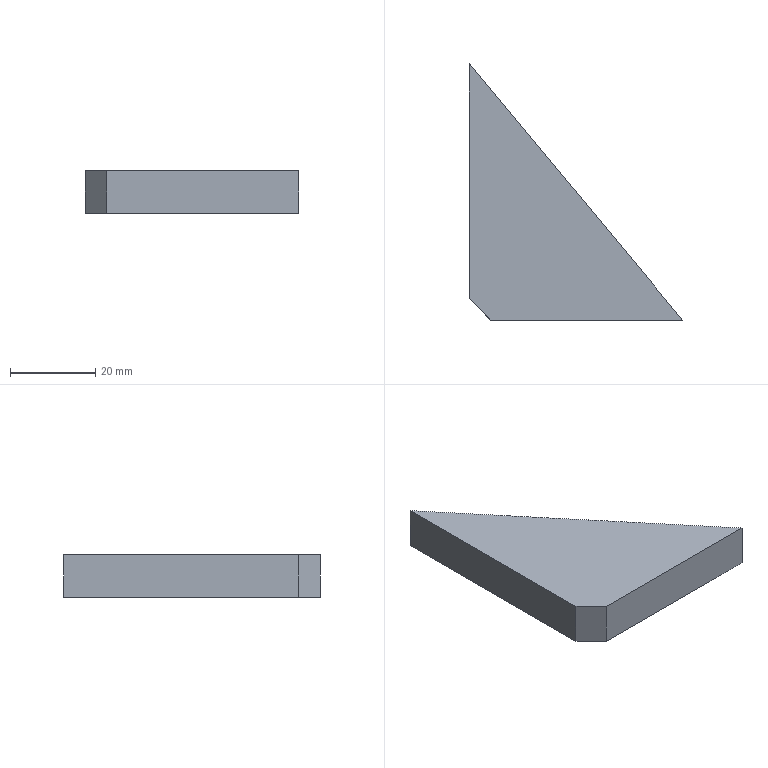Part | SolidWorks | features Chamfer 1, Extrusion 1 | 1 solid | 6 faces | box 50 x 60 x 10 mm | volume 14875 mm3 | plane 6
STEP:
#1=CARTESIAN_POINT('',(5.,0.,5.));
#2=VERTEX_POINT('',#1);
#3=CARTESIAN_POINT('',(50.,0.,5.));
#4=VERTEX_POINT('',#3);
#5=CARTESIAN_POINT('',(50.,0.,5.));
#6=DIRECTION('',(1.,0.,0.));
#7=VECTOR('',#6,1000.);
#8=LINE('',#5,#7);
#9=EDGE_CURVE('',#2,#4,#8,.T.);
#10=ORIENTED_EDGE('',*,*,#9,.F.);
#11=CARTESIAN_POINT('',(5.,0.,-5.));
#12=VERTEX_POINT('',#11);
#13=CARTESIAN_POINT('',(5.,0.,5.));
#14=DIRECTION('',(0.,0.,-1.));
#15=VECTOR('',#14,1000.);
#16=LINE('',#13,#15);
#17=EDGE_CURVE('',#2,#12,#16,.T.);
#18=ORIENTED_EDGE('',*,*,#17,.T.);
#19=CARTESIAN_POINT('',(50.,0.,-5.));
#20=VERTEX_POINT('',#19);
#21=CARTESIAN_POINT('',(50.,0.,-5.));
#22=DIRECTION('',(1.,0.,0.));
#23=VECTOR('',#22,1000.);
#24=LINE('',#21,#23);
#25=EDGE_CURVE('',#12,#20,#24,.T.);
#26=ORIENTED_EDGE('',*,*,#25,.T.);
#27=CARTESIAN_POINT('',(50.,0.,5.));
#28=DIRECTION('',(0.,0.,-1.));
#29=VECTOR('',#28,1000.);
#30=LINE('',#27,#29);
#31=EDGE_CURVE('',#4,#20,#30,.T.);
#32=ORIENTED_EDGE('',*,*,#31,.F.);
#33=EDGE_LOOP('',(#10,#18,#26,#32));
#34=FACE_OUTER_BOUND('',#33,.T.);
#35=CARTESIAN_POINT('',(50.,0.,5.));
#36=DIRECTION('',(0.,1.,0.));
#37=DIRECTION('',(0.,0.,1.));
#38=AXIS2_PLACEMENT_3D('',#35,#36,#37);
#39=PLANE('',#38);
#40=ADVANCED_FACE('',(#34),#39,.F.);
#41=CARTESIAN_POINT('',(0.,60.,-5.));
#42=VERTEX_POINT('',#41);
#43=CARTESIAN_POINT('',(0.,60.,-5.));
#44=DIRECTION('',(-0.6402,0.7682,0.));
#45=VECTOR('',#44,1000.);
#46=LINE('',#43,#45);
#47=EDGE_CURVE('',#20,#42,#46,.T.);
#48=ORIENTED_EDGE('',*,*,#47,.T.);
#49=CARTESIAN_POINT('',(0.,60.,5.));
#50=VERTEX_POINT('',#49);
#51=CARTESIAN_POINT('',(0.,60.,5.));
#52=DIRECTION('',(0.,0.,-1.));
#53=VECTOR('',#52,1000.);
#54=LINE('',#51,#53);
#55=EDGE_CURVE('',#50,#42,#54,.T.);
#56=ORIENTED_EDGE('',*,*,#55,.F.);
#57=CARTESIAN_POINT('',(0.,60.,5.));
#58=DIRECTION('',(-0.6402,0.7682,0.));
#59=VECTOR('',#58,1000.);
#60=LINE('',#57,#59);
#61=EDGE_CURVE('',#4,#50,#60,.T.);
#62=ORIENTED_EDGE('',*,*,#61,.F.);
#63=ORIENTED_EDGE('',*,*,#31,.T.);
#64=EDGE_LOOP('',(#48,#56,#62,#63));
#65=FACE_OUTER_BOUND('',#64,.T.);
#66=CARTESIAN_POINT('',(0.,60.,5.));
#67=DIRECTION('',(-0.7682,-0.6402,0.));
#68=DIRECTION('',(0.6402,-0.7682,0.));
#69=AXIS2_PLACEMENT_3D('',#66,#67,#68);
#70=PLANE('',#69);
#71=ADVANCED_FACE('',(#65),#70,.F.);
#72=CARTESIAN_POINT('',(0.,5.,-5.));
#73=VERTEX_POINT('',#72);
#74=CARTESIAN_POINT('',(0.,0.,-5.));
#75=DIRECTION('',(0.,-1.,0.));
#76=VECTOR('',#75,1000.);
#77=LINE('',#74,#76);
#78=EDGE_CURVE('',#42,#73,#77,.T.);
#79=ORIENTED_EDGE('',*,*,#78,.T.);
#80=CARTESIAN_POINT('',(0.,5.,5.));
#81=VERTEX_POINT('',#80);
#82=CARTESIAN_POINT('',(0.,5.,5.));
#83=DIRECTION('',(0.,0.,1.));
#84=VECTOR('',#83,1000.);
#85=LINE('',#82,#84);
#86=EDGE_CURVE('',#73,#81,#85,.T.);
#87=ORIENTED_EDGE('',*,*,#86,.T.);
#88=CARTESIAN_POINT('',(0.,0.,5.));
#89=DIRECTION('',(0.,-1.,0.));
#90=VECTOR('',#89,1000.);
#91=LINE('',#88,#90);
#92=EDGE_CURVE('',#50,#81,#91,.T.);
#93=ORIENTED_EDGE('',*,*,#92,.F.);
#94=ORIENTED_EDGE('',*,*,#55,.T.);
#95=EDGE_LOOP('',(#79,#87,#93,#94));
#96=FACE_OUTER_BOUND('',#95,.T.);
#97=CARTESIAN_POINT('',(0.,0.,5.));
#98=DIRECTION('',(1.,0.,0.));
#99=DIRECTION('',(0.,0.,-1.));
#100=AXIS2_PLACEMENT_3D('',#97,#98,#99);
#101=PLANE('',#100);
#102=ADVANCED_FACE('',(#96),#101,.F.);
#103=ORIENTED_EDGE('',*,*,#92,.T.);
#104=CARTESIAN_POINT('',(5.,0.,5.));
#105=DIRECTION('',(0.7071,-0.7071,0.));
#106=VECTOR('',#105,1000.);
#107=LINE('',#104,#106);
#108=EDGE_CURVE('',#81,#2,#107,.T.);
#109=ORIENTED_EDGE('',*,*,#108,.T.);
#110=ORIENTED_EDGE('',*,*,#9,.T.);
#111=ORIENTED_EDGE('',*,*,#61,.T.);
#112=EDGE_LOOP('',(#103,#109,#110,#111));
#113=FACE_OUTER_BOUND('',#112,.T.);
#114=CARTESIAN_POINT('',(0.,0.,5.));
#115=DIRECTION('',(0.,0.,-1.));
#116=DIRECTION('',(-1.,0.,0.));
#117=AXIS2_PLACEMENT_3D('',#114,#115,#116);
#118=PLANE('',#117);
#119=ADVANCED_FACE('',(#113),#118,.F.);
#120=ORIENTED_EDGE('',*,*,#25,.F.);
#121=CARTESIAN_POINT('',(2.5,2.5,-5.));
#122=DIRECTION('',(-0.7071,0.7071,0.));
#123=VECTOR('',#122,1000.);
#124=LINE('',#121,#123);
#125=EDGE_CURVE('',#12,#73,#124,.T.);
#126=ORIENTED_EDGE('',*,*,#125,.T.);
#127=ORIENTED_EDGE('',*,*,#78,.F.);
#128=ORIENTED_EDGE('',*,*,#47,.F.);
#129=EDGE_LOOP('',(#120,#126,#127,#128));
#130=FACE_OUTER_BOUND('',#129,.T.);
#131=CARTESIAN_POINT('',(0.,0.,-5.));
#132=DIRECTION('',(0.,0.,-1.));
#133=DIRECTION('',(-1.,0.,0.));
#134=AXIS2_PLACEMENT_3D('',#131,#132,#133);
#135=PLANE('',#134);
#136=ADVANCED_FACE('',(#130),#135,.T.);
#137=ORIENTED_EDGE('',*,*,#108,.F.);
#138=ORIENTED_EDGE('',*,*,#86,.F.);
#139=ORIENTED_EDGE('',*,*,#125,.F.);
#140=ORIENTED_EDGE('',*,*,#17,.F.);
#141=EDGE_LOOP('',(#137,#138,#139,#140));
#142=FACE_OUTER_BOUND('',#141,.T.);
#143=CARTESIAN_POINT('',(5.,0.,5.));
#144=DIRECTION('',(0.7071,0.7071,0.));
#145=DIRECTION('',(0.,0.,-1.));
#146=AXIS2_PLACEMENT_3D('',#143,#144,#145);
#147=PLANE('',#146);
#148=ADVANCED_FACE('',(#142),#147,.F.);
#149=CLOSED_SHELL('',(#40,#71,#102,#119,#136,#148));
#150=MANIFOLD_SOLID_BREP('',#149);
#151=CARTESIAN_POINT('',(0.,0.,0.));
#152=DIRECTION('',(0.,0.,1.));
#153=DIRECTION('',(1.,0.,0.));
#154=AXIS2_PLACEMENT_3D('',#151,#152,#153);
#155=(LENGTH_UNIT()NAMED_UNIT(*)SI_UNIT(.MILLI.,.METRE.));
#156=UNCERTAINTY_MEASURE_WITH_UNIT(LENGTH_MEASURE(0.00001),#155,'','');
#157=(NAMED_UNIT(*)PLANE_ANGLE_UNIT()SI_UNIT($,.RADIAN.));
#158=(NAMED_UNIT(*)SI_UNIT($,.STERADIAN.)SOLID_ANGLE_UNIT());
#159=(GEOMETRIC_REPRESENTATION_CONTEXT(3)GLOBAL_UNCERTAINTY_ASSIGNED_CONTEXT((#156))GLOBAL_UNIT_ASSIGNED_CONTEXT((#155,#157,#158))REPRESENTATION_CONTEXT('',''));
#160=ADVANCED_BREP_SHAPE_REPRESENTATION('',(#150,#154),#159);